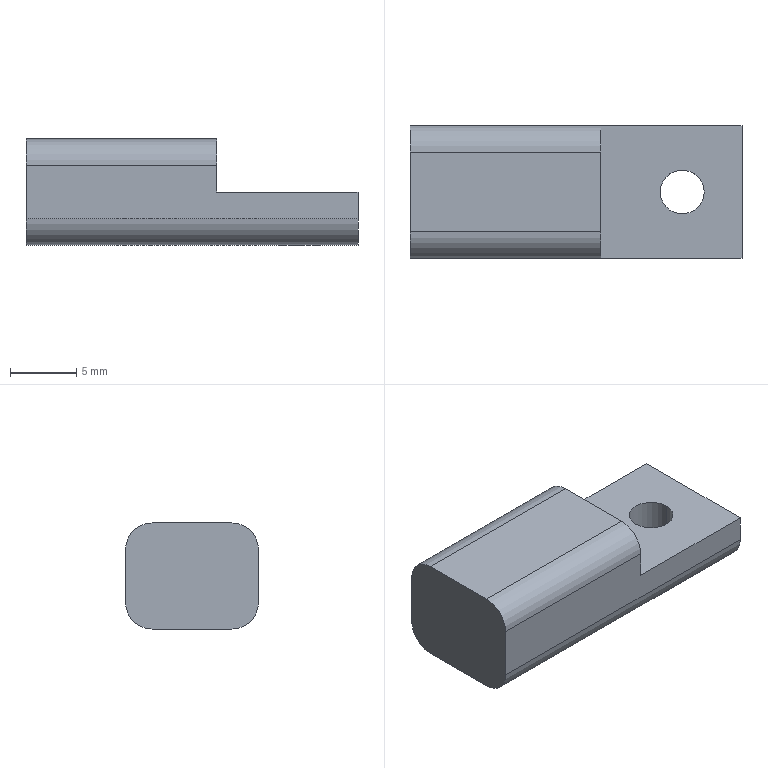Part | STEP file | 04-08 rotary limit block | 1 solid | 14 faces | box 25 x 10 x 8 mm | volume 1473 mm3 | plane 8 | cylinder 6 | commonest cylinder face diameters 4 x4 3.3 x2
STEP:
#1=CARTESIAN_POINT('',(6.35,0.,4.));
#2=VERTEX_POINT('',#1);
#3=CARTESIAN_POINT('',(9.65,0.,4.));
#4=VERTEX_POINT('',#3);
#5=CARTESIAN_POINT('',(8.,0.,4.));
#6=DIRECTION('',(0.,0.,1.));
#7=DIRECTION('',(-1.,0.,0.));
#8=AXIS2_PLACEMENT_3D('',#5,#6,#7);
#9=CIRCLE('',#8,1.65);
#10=EDGE_CURVE('',#2,#4,#9,.T.);
#11=ORIENTED_EDGE('',*,*,#10,.T.);
#12=CARTESIAN_POINT('',(9.65,0.,0.));
#13=VERTEX_POINT('',#12);
#14=CARTESIAN_POINT('',(9.65,0.,0.));
#15=DIRECTION('',(0.,0.,-1.));
#16=VECTOR('',#15,1000.);
#17=LINE('',#14,#16);
#18=EDGE_CURVE('',#4,#13,#17,.T.);
#19=ORIENTED_EDGE('',*,*,#18,.T.);
#20=CARTESIAN_POINT('',(6.35,0.,0.));
#21=VERTEX_POINT('',#20);
#22=CARTESIAN_POINT('',(8.,0.,0.));
#23=DIRECTION('',(0.,0.,-1.));
#24=DIRECTION('',(-1.,0.,0.));
#25=AXIS2_PLACEMENT_3D('',#22,#23,#24);
#26=CIRCLE('',#25,1.65);
#27=EDGE_CURVE('',#13,#21,#26,.T.);
#28=ORIENTED_EDGE('',*,*,#27,.T.);
#29=CARTESIAN_POINT('',(6.35,0.,0.));
#30=DIRECTION('',(0.,0.,-1.));
#31=VECTOR('',#30,1000.);
#32=LINE('',#29,#31);
#33=EDGE_CURVE('',#2,#21,#32,.T.);
#34=ORIENTED_EDGE('',*,*,#33,.F.);
#35=EDGE_LOOP('',(#11,#19,#28,#34));
#36=FACE_OUTER_BOUND('',#35,.T.);
#37=CARTESIAN_POINT('',(8.,0.,0.));
#38=DIRECTION('',(0.,0.,-1.));
#39=DIRECTION('',(-1.,0.,0.));
#40=AXIS2_PLACEMENT_3D('',#37,#38,#39);
#41=CYLINDRICAL_SURFACE('',#40,1.65);
#42=ADVANCED_FACE('',(#36),#41,.F.);
#43=CARTESIAN_POINT('',(12.5,5.,4.));
#44=VERTEX_POINT('',#43);
#45=CARTESIAN_POINT('',(12.5,5.,2.));
#46=VERTEX_POINT('',#45);
#47=CARTESIAN_POINT('',(12.5,5.,8.));
#48=DIRECTION('',(0.,0.,-1.));
#49=VECTOR('',#48,1000.);
#50=LINE('',#47,#49);
#51=EDGE_CURVE('',#44,#46,#50,.T.);
#52=ORIENTED_EDGE('',*,*,#51,.F.);
#53=CARTESIAN_POINT('',(12.5,-5.,4.));
#54=VERTEX_POINT('',#53);
#55=CARTESIAN_POINT('',(12.5,5.,4.));
#56=DIRECTION('',(0.,-1.,0.));
#57=VECTOR('',#56,1000.);
#58=LINE('',#55,#57);
#59=EDGE_CURVE('',#44,#54,#58,.T.);
#60=ORIENTED_EDGE('',*,*,#59,.T.);
#61=CARTESIAN_POINT('',(12.5,-5.,2.));
#62=VERTEX_POINT('',#61);
#63=CARTESIAN_POINT('',(12.5,-5.,8.));
#64=DIRECTION('',(0.,0.,-1.));
#65=VECTOR('',#64,1000.);
#66=LINE('',#63,#65);
#67=EDGE_CURVE('',#54,#62,#66,.T.);
#68=ORIENTED_EDGE('',*,*,#67,.T.);
#69=CARTESIAN_POINT('',(12.5,-3.,0.));
#70=VERTEX_POINT('',#69);
#71=CARTESIAN_POINT('',(12.5,-3.,2.));
#72=DIRECTION('',(1.,0.,0.));
#73=DIRECTION('',(0.,-1.,0.));
#74=AXIS2_PLACEMENT_3D('',#71,#72,#73);
#75=CIRCLE('',#74,2.);
#76=EDGE_CURVE('',#62,#70,#75,.T.);
#77=ORIENTED_EDGE('',*,*,#76,.T.);
#78=CARTESIAN_POINT('',(12.5,3.,0.));
#79=VERTEX_POINT('',#78);
#80=CARTESIAN_POINT('',(12.5,5.,0.));
#81=DIRECTION('',(0.,1.,0.));
#82=VECTOR('',#81,1000.);
#83=LINE('',#80,#82);
#84=EDGE_CURVE('',#70,#79,#83,.T.);
#85=ORIENTED_EDGE('',*,*,#84,.T.);
#86=CARTESIAN_POINT('',(12.5,3.,2.));
#87=DIRECTION('',(1.,0.,0.));
#88=DIRECTION('',(0.,-1.,0.));
#89=AXIS2_PLACEMENT_3D('',#86,#87,#88);
#90=CIRCLE('',#89,2.);
#91=EDGE_CURVE('',#79,#46,#90,.T.);
#92=ORIENTED_EDGE('',*,*,#91,.T.);
#93=EDGE_LOOP('',(#52,#60,#68,#77,#85,#92));
#94=FACE_OUTER_BOUND('',#93,.T.);
#95=CARTESIAN_POINT('',(12.5,5.,8.));
#96=DIRECTION('',(-1.,0.,0.));
#97=DIRECTION('',(0.,-1.,0.));
#98=AXIS2_PLACEMENT_3D('',#95,#96,#97);
#99=PLANE('',#98);
#100=ADVANCED_FACE('',(#94),#99,.F.);
#101=CARTESIAN_POINT('',(1.879,5.,6.));
#102=VERTEX_POINT('',#101);
#103=CARTESIAN_POINT('',(1.879,5.,4.));
#104=VERTEX_POINT('',#103);
#105=CARTESIAN_POINT('',(1.879,5.,8.));
#106=DIRECTION('',(0.,0.,-1.));
#107=VECTOR('',#106,1000.);
#108=LINE('',#105,#107);
#109=EDGE_CURVE('',#102,#104,#108,.T.);
#110=ORIENTED_EDGE('',*,*,#109,.T.);
#111=CARTESIAN_POINT('',(12.5,5.,4.));
#112=DIRECTION('',(1.,0.,0.));
#113=VECTOR('',#112,1000.);
#114=LINE('',#111,#113);
#115=EDGE_CURVE('',#104,#44,#114,.T.);
#116=ORIENTED_EDGE('',*,*,#115,.T.);
#117=ORIENTED_EDGE('',*,*,#51,.T.);
#118=CARTESIAN_POINT('',(-12.5,5.,2.));
#119=VERTEX_POINT('',#118);
#120=CARTESIAN_POINT('',(-12.5,5.,2.));
#121=DIRECTION('',(-1.,0.,0.));
#122=VECTOR('',#121,1000.);
#123=LINE('',#120,#122);
#124=EDGE_CURVE('',#46,#119,#123,.T.);
#125=ORIENTED_EDGE('',*,*,#124,.T.);
#126=CARTESIAN_POINT('',(-12.5,5.,6.));
#127=VERTEX_POINT('',#126);
#128=CARTESIAN_POINT('',(-12.5,5.,8.));
#129=DIRECTION('',(0.,0.,-1.));
#130=VECTOR('',#129,1000.);
#131=LINE('',#128,#130);
#132=EDGE_CURVE('',#127,#119,#131,.T.);
#133=ORIENTED_EDGE('',*,*,#132,.F.);
#134=CARTESIAN_POINT('',(12.5,5.,6.));
#135=DIRECTION('',(1.,0.,0.));
#136=VECTOR('',#135,1000.);
#137=LINE('',#134,#136);
#138=EDGE_CURVE('',#127,#102,#137,.T.);
#139=ORIENTED_EDGE('',*,*,#138,.T.);
#140=EDGE_LOOP('',(#110,#116,#117,#125,#133,#139));
#141=FACE_OUTER_BOUND('',#140,.T.);
#142=CARTESIAN_POINT('',(-12.5,5.,8.));
#143=DIRECTION('',(0.,-1.,0.));
#144=DIRECTION('',(0.,0.,-1.));
#145=AXIS2_PLACEMENT_3D('',#142,#143,#144);
#146=PLANE('',#145);
#147=ADVANCED_FACE('',(#141),#146,.F.);
#148=CARTESIAN_POINT('',(-12.5,3.,0.));
#149=VERTEX_POINT('',#148);
#150=CARTESIAN_POINT('',(-12.5,-3.,0.));
#151=VERTEX_POINT('',#150);
#152=CARTESIAN_POINT('',(-12.5,5.,0.));
#153=DIRECTION('',(0.,-1.,0.));
#154=VECTOR('',#153,1000.);
#155=LINE('',#152,#154);
#156=EDGE_CURVE('',#149,#151,#155,.T.);
#157=ORIENTED_EDGE('',*,*,#156,.T.);
#158=CARTESIAN_POINT('',(-12.5,-5.,2.));
#159=VERTEX_POINT('',#158);
#160=CARTESIAN_POINT('',(-12.5,-3.,2.));
#161=DIRECTION('',(-1.,0.,0.));
#162=DIRECTION('',(0.,1.,0.));
#163=AXIS2_PLACEMENT_3D('',#160,#161,#162);
#164=CIRCLE('',#163,2.);
#165=EDGE_CURVE('',#151,#159,#164,.T.);
#166=ORIENTED_EDGE('',*,*,#165,.T.);
#167=CARTESIAN_POINT('',(-12.5,-5.,6.));
#168=VERTEX_POINT('',#167);
#169=CARTESIAN_POINT('',(-12.5,-5.,8.));
#170=DIRECTION('',(0.,0.,-1.));
#171=VECTOR('',#170,1000.);
#172=LINE('',#169,#171);
#173=EDGE_CURVE('',#168,#159,#172,.T.);
#174=ORIENTED_EDGE('',*,*,#173,.F.);
#175=CARTESIAN_POINT('',(-12.5,-3.,8.));
#176=VERTEX_POINT('',#175);
#177=CARTESIAN_POINT('',(-12.5,-3.,6.));
#178=DIRECTION('',(-1.,0.,0.));
#179=DIRECTION('',(0.,1.,0.));
#180=AXIS2_PLACEMENT_3D('',#177,#178,#179);
#181=CIRCLE('',#180,2.);
#182=EDGE_CURVE('',#168,#176,#181,.T.);
#183=ORIENTED_EDGE('',*,*,#182,.T.);
#184=CARTESIAN_POINT('',(-12.5,3.,8.));
#185=VERTEX_POINT('',#184);
#186=CARTESIAN_POINT('',(-12.5,5.,8.));
#187=DIRECTION('',(0.,-1.,0.));
#188=VECTOR('',#187,1000.);
#189=LINE('',#186,#188);
#190=EDGE_CURVE('',#185,#176,#189,.T.);
#191=ORIENTED_EDGE('',*,*,#190,.F.);
#192=CARTESIAN_POINT('',(-12.5,3.,6.));
#193=DIRECTION('',(-1.,0.,0.));
#194=DIRECTION('',(0.,1.,0.));
#195=AXIS2_PLACEMENT_3D('',#192,#193,#194);
#196=CIRCLE('',#195,2.);
#197=EDGE_CURVE('',#185,#127,#196,.T.);
#198=ORIENTED_EDGE('',*,*,#197,.T.);
#199=ORIENTED_EDGE('',*,*,#132,.T.);
#200=CARTESIAN_POINT('',(-12.5,3.,2.));
#201=DIRECTION('',(-1.,0.,0.));
#202=DIRECTION('',(0.,1.,0.));
#203=AXIS2_PLACEMENT_3D('',#200,#201,#202);
#204=CIRCLE('',#203,2.);
#205=EDGE_CURVE('',#119,#149,#204,.T.);
#206=ORIENTED_EDGE('',*,*,#205,.T.);
#207=EDGE_LOOP('',(#157,#166,#174,#183,#191,#198,#199,#206));
#208=FACE_OUTER_BOUND('',#207,.T.);
#209=CARTESIAN_POINT('',(-12.5,5.,8.));
#210=DIRECTION('',(1.,0.,0.));
#211=DIRECTION('',(0.,1.,0.));
#212=AXIS2_PLACEMENT_3D('',#209,#210,#211);
#213=PLANE('',#212);
#214=ADVANCED_FACE('',(#208),#213,.F.);
#215=ORIENTED_EDGE('',*,*,#67,.F.);
#216=CARTESIAN_POINT('',(1.879,-5.,4.));
#217=VERTEX_POINT('',#216);
#218=CARTESIAN_POINT('',(12.5,-5.,4.));
#219=DIRECTION('',(1.,0.,0.));
#220=VECTOR('',#219,1000.);
#221=LINE('',#218,#220);
#222=EDGE_CURVE('',#217,#54,#221,.T.);
#223=ORIENTED_EDGE('',*,*,#222,.F.);
#224=CARTESIAN_POINT('',(1.879,-5.,6.));
#225=VERTEX_POINT('',#224);
#226=CARTESIAN_POINT('',(1.879,-5.,8.));
#227=DIRECTION('',(0.,0.,-1.));
#228=VECTOR('',#227,1000.);
#229=LINE('',#226,#228);
#230=EDGE_CURVE('',#225,#217,#229,.T.);
#231=ORIENTED_EDGE('',*,*,#230,.F.);
#232=CARTESIAN_POINT('',(-12.5,-5.,6.));
#233=DIRECTION('',(-1.,0.,0.));
#234=VECTOR('',#233,1000.);
#235=LINE('',#232,#234);
#236=EDGE_CURVE('',#225,#168,#235,.T.);
#237=ORIENTED_EDGE('',*,*,#236,.T.);
#238=ORIENTED_EDGE('',*,*,#173,.T.);
#239=CARTESIAN_POINT('',(-12.5,-5.,2.));
#240=DIRECTION('',(1.,0.,0.));
#241=VECTOR('',#240,1000.);
#242=LINE('',#239,#241);
#243=EDGE_CURVE('',#159,#62,#242,.T.);
#244=ORIENTED_EDGE('',*,*,#243,.T.);
#245=EDGE_LOOP('',(#215,#223,#231,#237,#238,#244));
#246=FACE_OUTER_BOUND('',#245,.T.);
#247=CARTESIAN_POINT('',(-12.5,-5.,8.));
#248=DIRECTION('',(0.,1.,0.));
#249=DIRECTION('',(0.,0.,1.));
#250=AXIS2_PLACEMENT_3D('',#247,#248,#249);
#251=PLANE('',#250);
#252=ADVANCED_FACE('',(#246),#251,.F.);
#253=CARTESIAN_POINT('',(1.879,3.,8.));
#254=VERTEX_POINT('',#253);
#255=CARTESIAN_POINT('',(1.879,-3.,8.));
#256=VERTEX_POINT('',#255);
#257=CARTESIAN_POINT('',(1.879,5.,8.));
#258=DIRECTION('',(0.,-1.,0.));
#259=VECTOR('',#258,1000.);
#260=LINE('',#257,#259);
#261=EDGE_CURVE('',#254,#256,#260,.T.);
#262=ORIENTED_EDGE('',*,*,#261,.F.);
#263=CARTESIAN_POINT('',(-12.5,3.,8.));
#264=DIRECTION('',(-1.,0.,0.));
#265=VECTOR('',#264,1000.);
#266=LINE('',#263,#265);
#267=EDGE_CURVE('',#254,#185,#266,.T.);
#268=ORIENTED_EDGE('',*,*,#267,.T.);
#269=ORIENTED_EDGE('',*,*,#190,.T.);
#270=CARTESIAN_POINT('',(12.5,-3.,8.));
#271=DIRECTION('',(1.,0.,0.));
#272=VECTOR('',#271,1000.);
#273=LINE('',#270,#272);
#274=EDGE_CURVE('',#176,#256,#273,.T.);
#275=ORIENTED_EDGE('',*,*,#274,.T.);
#276=EDGE_LOOP('',(#262,#268,#269,#275));
#277=FACE_OUTER_BOUND('',#276,.T.);
#278=CARTESIAN_POINT('',(12.5,-5.,8.));
#279=DIRECTION('',(0.,0.,1.));
#280=DIRECTION('',(1.,0.,0.));
#281=AXIS2_PLACEMENT_3D('',#278,#279,#280);
#282=PLANE('',#281);
#283=ADVANCED_FACE('',(#277),#282,.T.);
#284=CARTESIAN_POINT('',(8.,0.,0.));
#285=DIRECTION('',(0.,0.,-1.));
#286=DIRECTION('',(-1.,0.,0.));
#287=AXIS2_PLACEMENT_3D('',#284,#285,#286);
#288=CIRCLE('',#287,1.65);
#289=EDGE_CURVE('',#21,#13,#288,.T.);
#290=ORIENTED_EDGE('',*,*,#289,.F.);
#291=ORIENTED_EDGE('',*,*,#27,.F.);
#292=EDGE_LOOP('',(#290,#291));
#293=FACE_BOUND('',#292,.T.);
#294=ORIENTED_EDGE('',*,*,#84,.F.);
#295=CARTESIAN_POINT('',(12.5,-3.,0.));
#296=DIRECTION('',(-1.,0.,0.));
#297=VECTOR('',#296,1000.);
#298=LINE('',#295,#297);
#299=EDGE_CURVE('',#70,#151,#298,.T.);
#300=ORIENTED_EDGE('',*,*,#299,.T.);
#301=ORIENTED_EDGE('',*,*,#156,.F.);
#302=CARTESIAN_POINT('',(12.5,3.,0.));
#303=DIRECTION('',(1.,0.,0.));
#304=VECTOR('',#303,1000.);
#305=LINE('',#302,#304);
#306=EDGE_CURVE('',#149,#79,#305,.T.);
#307=ORIENTED_EDGE('',*,*,#306,.T.);
#308=EDGE_LOOP('',(#294,#300,#301,#307));
#309=FACE_OUTER_BOUND('',#308,.T.);
#310=CARTESIAN_POINT('',(12.5,-5.,0.));
#311=DIRECTION('',(0.,0.,1.));
#312=DIRECTION('',(1.,0.,0.));
#313=AXIS2_PLACEMENT_3D('',#310,#311,#312);
#314=PLANE('',#313);
#315=ADVANCED_FACE('',(#293,#309),#314,.F.);
#316=ORIENTED_EDGE('',*,*,#18,.F.);
#317=CARTESIAN_POINT('',(8.,0.,4.));
#318=DIRECTION('',(0.,0.,1.));
#319=DIRECTION('',(-1.,0.,0.));
#320=AXIS2_PLACEMENT_3D('',#317,#318,#319);
#321=CIRCLE('',#320,1.65);
#322=EDGE_CURVE('',#4,#2,#321,.T.);
#323=ORIENTED_EDGE('',*,*,#322,.T.);
#324=ORIENTED_EDGE('',*,*,#33,.T.);
#325=ORIENTED_EDGE('',*,*,#289,.T.);
#326=EDGE_LOOP('',(#316,#323,#324,#325));
#327=FACE_OUTER_BOUND('',#326,.T.);
#328=CARTESIAN_POINT('',(8.,0.,0.));
#329=DIRECTION('',(0.,0.,-1.));
#330=DIRECTION('',(-1.,0.,0.));
#331=AXIS2_PLACEMENT_3D('',#328,#329,#330);
#332=CYLINDRICAL_SURFACE('',#331,1.65);
#333=ADVANCED_FACE('',(#327),#332,.F.);
#334=ORIENTED_EDGE('',*,*,#165,.F.);
#335=ORIENTED_EDGE('',*,*,#299,.F.);
#336=ORIENTED_EDGE('',*,*,#76,.F.);
#337=ORIENTED_EDGE('',*,*,#243,.F.);
#338=EDGE_LOOP('',(#334,#335,#336,#337));
#339=FACE_OUTER_BOUND('',#338,.T.);
#340=CARTESIAN_POINT('',(-12.5,-3.,2.));
#341=DIRECTION('',(1.,0.,0.));
#342=DIRECTION('',(0.,0.,-1.));
#343=AXIS2_PLACEMENT_3D('',#340,#341,#342);
#344=CYLINDRICAL_SURFACE('',#343,2.);
#345=ADVANCED_FACE('',(#339),#344,.T.);
#346=CARTESIAN_POINT('',(1.879,-3.,6.));
#347=DIRECTION('',(1.,0.,0.));
#348=DIRECTION('',(0.,0.,1.));
#349=AXIS2_PLACEMENT_3D('',#346,#347,#348);
#350=CIRCLE('',#349,2.);
#351=EDGE_CURVE('',#256,#225,#350,.T.);
#352=ORIENTED_EDGE('',*,*,#351,.F.);
#353=ORIENTED_EDGE('',*,*,#274,.F.);
#354=ORIENTED_EDGE('',*,*,#182,.F.);
#355=ORIENTED_EDGE('',*,*,#236,.F.);
#356=EDGE_LOOP('',(#352,#353,#354,#355));
#357=FACE_OUTER_BOUND('',#356,.T.);
#358=CARTESIAN_POINT('',(12.5,-3.,6.));
#359=DIRECTION('',(-1.,0.,0.));
#360=DIRECTION('',(0.,0.,1.));
#361=AXIS2_PLACEMENT_3D('',#358,#359,#360);
#362=CYLINDRICAL_SURFACE('',#361,2.);
#363=ADVANCED_FACE('',(#357),#362,.T.);
#364=CARTESIAN_POINT('',(1.879,3.,6.));
#365=DIRECTION('',(1.,0.,0.));
#366=DIRECTION('',(0.,0.,1.));
#367=AXIS2_PLACEMENT_3D('',#364,#365,#366);
#368=CIRCLE('',#367,2.);
#369=EDGE_CURVE('',#102,#254,#368,.T.);
#370=ORIENTED_EDGE('',*,*,#369,.F.);
#371=ORIENTED_EDGE('',*,*,#138,.F.);
#372=ORIENTED_EDGE('',*,*,#197,.F.);
#373=ORIENTED_EDGE('',*,*,#267,.F.);
#374=EDGE_LOOP('',(#370,#371,#372,#373));
#375=FACE_OUTER_BOUND('',#374,.T.);
#376=CARTESIAN_POINT('',(12.5,3.,6.));
#377=DIRECTION('',(1.,0.,0.));
#378=DIRECTION('',(0.,0.,-1.));
#379=AXIS2_PLACEMENT_3D('',#376,#377,#378);
#380=CYLINDRICAL_SURFACE('',#379,2.);
#381=ADVANCED_FACE('',(#375),#380,.T.);
#382=ORIENTED_EDGE('',*,*,#91,.F.);
#383=ORIENTED_EDGE('',*,*,#306,.F.);
#384=ORIENTED_EDGE('',*,*,#205,.F.);
#385=ORIENTED_EDGE('',*,*,#124,.F.);
#386=EDGE_LOOP('',(#382,#383,#384,#385));
#387=FACE_OUTER_BOUND('',#386,.T.);
#388=CARTESIAN_POINT('',(-12.5,3.,2.));
#389=DIRECTION('',(-1.,0.,0.));
#390=DIRECTION('',(0.,0.,1.));
#391=AXIS2_PLACEMENT_3D('',#388,#389,#390);
#392=CYLINDRICAL_SURFACE('',#391,2.);
#393=ADVANCED_FACE('',(#387),#392,.T.);
#394=ORIENTED_EDGE('',*,*,#222,.T.);
#395=ORIENTED_EDGE('',*,*,#59,.F.);
#396=ORIENTED_EDGE('',*,*,#115,.F.);
#397=CARTESIAN_POINT('',(1.879,5.,4.));
#398=DIRECTION('',(0.,-1.,0.));
#399=VECTOR('',#398,1000.);
#400=LINE('',#397,#399);
#401=EDGE_CURVE('',#104,#217,#400,.T.);
#402=ORIENTED_EDGE('',*,*,#401,.T.);
#403=EDGE_LOOP('',(#394,#395,#396,#402));
#404=FACE_OUTER_BOUND('',#403,.T.);
#405=ORIENTED_EDGE('',*,*,#10,.F.);
#406=ORIENTED_EDGE('',*,*,#322,.F.);
#407=EDGE_LOOP('',(#405,#406));
#408=FACE_BOUND('',#407,.T.);
#409=CARTESIAN_POINT('',(12.5,5.,4.));
#410=DIRECTION('',(0.,0.,-1.));
#411=DIRECTION('',(-1.,0.,0.));
#412=AXIS2_PLACEMENT_3D('',#409,#410,#411);
#413=PLANE('',#412);
#414=ADVANCED_FACE('',(#404,#408),#413,.F.);
#415=ORIENTED_EDGE('',*,*,#351,.T.);
#416=ORIENTED_EDGE('',*,*,#230,.T.);
#417=ORIENTED_EDGE('',*,*,#401,.F.);
#418=ORIENTED_EDGE('',*,*,#109,.F.);
#419=ORIENTED_EDGE('',*,*,#369,.T.);
#420=ORIENTED_EDGE('',*,*,#261,.T.);
#421=EDGE_LOOP('',(#415,#416,#417,#418,#419,#420));
#422=FACE_OUTER_BOUND('',#421,.T.);
#423=CARTESIAN_POINT('',(1.879,5.,8.));
#424=DIRECTION('',(-1.,0.,0.));
#425=DIRECTION('',(0.,0.,1.));
#426=AXIS2_PLACEMENT_3D('',#423,#424,#425);
#427=PLANE('',#426);
#428=ADVANCED_FACE('',(#422),#427,.F.);
#429=CLOSED_SHELL('',(#42,#100,#147,#214,#252,#283,#315,#333,#345,#363,#381,#393,#414,#428));
#430=MANIFOLD_SOLID_BREP('',#429);
#431=CARTESIAN_POINT('',(0.,0.,0.));
#432=DIRECTION('',(0.,0.,1.));
#433=DIRECTION('',(1.,0.,0.));
#434=AXIS2_PLACEMENT_3D('',#431,#432,#433);
#435=(LENGTH_UNIT()NAMED_UNIT(*)SI_UNIT(.MILLI.,.METRE.));
#436=UNCERTAINTY_MEASURE_WITH_UNIT(LENGTH_MEASURE(0.00001),#435,'','');
#437=(NAMED_UNIT(*)PLANE_ANGLE_UNIT()SI_UNIT($,.RADIAN.));
#438=(NAMED_UNIT(*)SI_UNIT($,.STERADIAN.)SOLID_ANGLE_UNIT());
#439=(GEOMETRIC_REPRESENTATION_CONTEXT(3)GLOBAL_UNCERTAINTY_ASSIGNED_CONTEXT((#436))GLOBAL_UNIT_ASSIGNED_CONTEXT((#435,#437,#438))REPRESENTATION_CONTEXT('',''));
#440=ADVANCED_BREP_SHAPE_REPRESENTATION('',(#430,#434),#439);